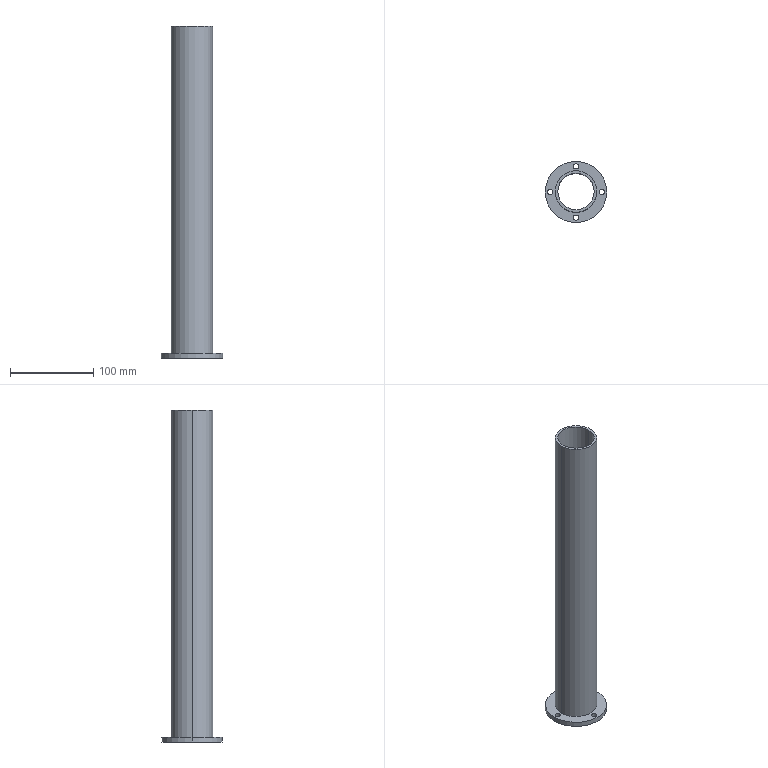Part | STEP file | QA-TE01 | 1 solid | 17 faces | box 74 x 74 x 400 mm | volume 190414 mm3 | cylinder 14 | plane 3 | commonest cylinder face diameters 6.5 x8 44 x2 50 x2 74 x2
STEP:
#1=CARTESIAN_POINT('',(0.,0.,0.));
#2=DIRECTION('',(0.,0.,1.));
#3=DIRECTION('',(1.,0.,0.));
#4=AXIS2_PLACEMENT_3D('',#1,#2,#3);
#5=CARTESIAN_POINT('',(22.,0.,0.));
#6=VERTEX_POINT('',#5);
#7=CARTESIAN_POINT('',(22.,0.,400.));
#8=VERTEX_POINT('',#7);
#9=CARTESIAN_POINT('',(22.,0.,0.));
#10=DIRECTION('',(0.,0.,1.));
#11=VECTOR('',#10,1.);
#12=LINE('',#9,#11);
#13=CARTESIAN_POINT('',(0.,0.,0.));
#14=DIRECTION('',(0.,0.,1.));
#15=DIRECTION('',(1.,0.,0.));
#16=AXIS2_PLACEMENT_3D('',#13,#14,#15);
#17=CYLINDRICAL_SURFACE('',#16,22.);
#18=CARTESIAN_POINT('',(6.283,0.));
#19=DIRECTION('',(0.,1.));
#20=VECTOR('',#19,1.);
#21=LINE('',#18,#20);
#22=(GEOMETRIC_REPRESENTATION_CONTEXT(2)PARAMETRIC_REPRESENTATION_CONTEXT()REPRESENTATION_CONTEXT('',''));
#23=DEFINITIONAL_REPRESENTATION('',(#21),#22);
#24=PCURVE('',#17,#23);
#25=CARTESIAN_POINT('',(0.,0.,0.));
#26=DIRECTION('',(0.,0.,1.));
#27=DIRECTION('',(1.,0.,0.));
#28=AXIS2_PLACEMENT_3D('',#25,#26,#27);
#29=CYLINDRICAL_SURFACE('',#28,22.);
#30=CARTESIAN_POINT('',(0.,0.));
#31=DIRECTION('',(0.,1.));
#32=VECTOR('',#31,1.);
#33=LINE('',#30,#32);
#34=(GEOMETRIC_REPRESENTATION_CONTEXT(2)PARAMETRIC_REPRESENTATION_CONTEXT()REPRESENTATION_CONTEXT('',''));
#35=DEFINITIONAL_REPRESENTATION('',(#33),#34);
#36=PCURVE('',#29,#35);
#37=SURFACE_CURVE('',#12,(#24,#36),.PCURVE_S1.);
#38=EDGE_CURVE('',#6,#8,#37,.T.);
#39=ORIENTED_EDGE('',*,*,#38,.T.);
#40=CARTESIAN_POINT('',(-22.,0.,400.));
#41=VERTEX_POINT('',#40);
#42=CARTESIAN_POINT('',(0.,0.,400.));
#43=DIRECTION('',(0.,0.,1.));
#44=DIRECTION('',(1.,0.,0.));
#45=AXIS2_PLACEMENT_3D('',#42,#43,#44);
#46=CIRCLE('',#45,22.);
#47=CARTESIAN_POINT('',(0.,400.));
#48=DIRECTION('',(1.,0.));
#49=VECTOR('',#48,1.);
#50=LINE('',#47,#49);
#51=(GEOMETRIC_REPRESENTATION_CONTEXT(2)PARAMETRIC_REPRESENTATION_CONTEXT()REPRESENTATION_CONTEXT('',''));
#52=DEFINITIONAL_REPRESENTATION('',(#50),#51);
#53=PCURVE('',#17,#52);
#54=CARTESIAN_POINT('',(0.,0.,400.));
#55=DIRECTION('',(0.,0.,1.));
#56=DIRECTION('',(1.,0.,0.));
#57=AXIS2_PLACEMENT_3D('',#54,#55,#56);
#58=PLANE('',#57);
#59=CARTESIAN_POINT('',(0.,0.));
#60=DIRECTION('',(1.,0.));
#61=AXIS2_PLACEMENT_2D('',#59,#60);
#62=CIRCLE('',#61,22.);
#63=(GEOMETRIC_REPRESENTATION_CONTEXT(2)PARAMETRIC_REPRESENTATION_CONTEXT()REPRESENTATION_CONTEXT('',''));
#64=DEFINITIONAL_REPRESENTATION('',(#62),#63);
#65=PCURVE('',#58,#64);
#66=SURFACE_CURVE('',#46,(#53,#65),.PCURVE_S1.);
#67=EDGE_CURVE('',#41,#8,#66,.T.);
#68=ORIENTED_EDGE('',*,*,#67,.F.);
#69=CARTESIAN_POINT('',(-22.,0.,0.));
#70=VERTEX_POINT('',#69);
#71=CARTESIAN_POINT('',(-22.,0.,0.));
#72=DIRECTION('',(0.,0.,1.));
#73=VECTOR('',#72,1.);
#74=LINE('',#71,#73);
#75=CARTESIAN_POINT('',(3.142,0.));
#76=DIRECTION('',(0.,1.));
#77=VECTOR('',#76,1.);
#78=LINE('',#75,#77);
#79=(GEOMETRIC_REPRESENTATION_CONTEXT(2)PARAMETRIC_REPRESENTATION_CONTEXT()REPRESENTATION_CONTEXT('',''));
#80=DEFINITIONAL_REPRESENTATION('',(#78),#79);
#81=PCURVE('',#17,#80);
#82=CARTESIAN_POINT('',(3.142,0.));
#83=DIRECTION('',(0.,1.));
#84=VECTOR('',#83,1.);
#85=LINE('',#82,#84);
#86=(GEOMETRIC_REPRESENTATION_CONTEXT(2)PARAMETRIC_REPRESENTATION_CONTEXT()REPRESENTATION_CONTEXT('',''));
#87=DEFINITIONAL_REPRESENTATION('',(#85),#86);
#88=PCURVE('',#29,#87);
#89=SURFACE_CURVE('',#74,(#81,#88),.PCURVE_S1.);
#90=EDGE_CURVE('',#70,#41,#89,.T.);
#91=ORIENTED_EDGE('',*,*,#90,.F.);
#92=CARTESIAN_POINT('',(0.,0.,0.));
#93=DIRECTION('',(0.,0.,1.));
#94=DIRECTION('',(1.,0.,0.));
#95=AXIS2_PLACEMENT_3D('',#92,#93,#94);
#96=CIRCLE('',#95,22.);
#97=CARTESIAN_POINT('',(0.,0.));
#98=DIRECTION('',(1.,0.));
#99=VECTOR('',#98,1.);
#100=LINE('',#97,#99);
#101=(GEOMETRIC_REPRESENTATION_CONTEXT(2)PARAMETRIC_REPRESENTATION_CONTEXT()REPRESENTATION_CONTEXT('',''));
#102=DEFINITIONAL_REPRESENTATION('',(#100),#101);
#103=PCURVE('',#17,#102);
#104=CARTESIAN_POINT('',(0.,0.,0.));
#105=DIRECTION('',(0.,0.,1.));
#106=DIRECTION('',(1.,0.,0.));
#107=AXIS2_PLACEMENT_3D('',#104,#105,#106);
#108=PLANE('',#107);
#109=CARTESIAN_POINT('',(0.,0.));
#110=DIRECTION('',(1.,0.));
#111=AXIS2_PLACEMENT_2D('',#109,#110);
#112=CIRCLE('',#111,22.);
#113=(GEOMETRIC_REPRESENTATION_CONTEXT(2)PARAMETRIC_REPRESENTATION_CONTEXT()REPRESENTATION_CONTEXT('',''));
#114=DEFINITIONAL_REPRESENTATION('',(#112),#113);
#115=PCURVE('',#108,#114);
#116=SURFACE_CURVE('',#96,(#103,#115),.PCURVE_S1.);
#117=EDGE_CURVE('',#70,#6,#116,.T.);
#118=ORIENTED_EDGE('',*,*,#117,.T.);
#119=EDGE_LOOP('',(#39,#68,#91,#118));
#120=FACE_BOUND('',#119,.F.);
#121=ADVANCED_FACE('',(#120),#17,.F.);
#122=CARTESIAN_POINT('',(-34.25,0.,6.));
#123=VERTEX_POINT('',#122);
#124=CARTESIAN_POINT('',(-34.25,0.,0.));
#125=VERTEX_POINT('',#124);
#126=CARTESIAN_POINT('',(-34.25,0.,10.));
#127=DIRECTION('',(0.,0.,-1.));
#128=VECTOR('',#127,1.);
#129=LINE('',#126,#128);
#130=CARTESIAN_POINT('',(-31.,0.,10.));
#131=DIRECTION('',(0.,0.,-1.));
#132=DIRECTION('',(-1.,0.,0.));
#133=AXIS2_PLACEMENT_3D('',#130,#131,#132);
#134=CYLINDRICAL_SURFACE('',#133,3.25);
#135=CARTESIAN_POINT('',(6.283,0.));
#136=DIRECTION('',(0.,1.));
#137=VECTOR('',#136,1.);
#138=LINE('',#135,#137);
#139=(GEOMETRIC_REPRESENTATION_CONTEXT(2)PARAMETRIC_REPRESENTATION_CONTEXT()REPRESENTATION_CONTEXT('',''));
#140=DEFINITIONAL_REPRESENTATION('',(#138),#139);
#141=PCURVE('',#134,#140);
#142=CARTESIAN_POINT('',(-31.,0.,10.));
#143=DIRECTION('',(0.,0.,-1.));
#144=DIRECTION('',(-1.,0.,0.));
#145=AXIS2_PLACEMENT_3D('',#142,#143,#144);
#146=CYLINDRICAL_SURFACE('',#145,3.25);
#147=CARTESIAN_POINT('',(0.,0.));
#148=DIRECTION('',(0.,1.));
#149=VECTOR('',#148,1.);
#150=LINE('',#147,#149);
#151=(GEOMETRIC_REPRESENTATION_CONTEXT(2)PARAMETRIC_REPRESENTATION_CONTEXT()REPRESENTATION_CONTEXT('',''));
#152=DEFINITIONAL_REPRESENTATION('',(#150),#151);
#153=PCURVE('',#146,#152);
#154=SURFACE_CURVE('',#129,(#141,#153),.PCURVE_S1.);
#155=EDGE_CURVE('',#123,#125,#154,.T.);
#156=ORIENTED_EDGE('',*,*,#155,.T.);
#157=CARTESIAN_POINT('',(-27.75,0.,0.));
#158=VERTEX_POINT('',#157);
#159=CARTESIAN_POINT('',(-31.,0.,0.));
#160=DIRECTION('',(0.,0.,-1.));
#161=DIRECTION('',(0.,-1.,0.));
#162=AXIS2_PLACEMENT_3D('',#159,#160,#161);
#163=CIRCLE('',#162,3.25);
#164=CARTESIAN_POINT('',(-1.571,10.));
#165=DIRECTION('',(1.,0.));
#166=VECTOR('',#165,1.);
#167=LINE('',#164,#166);
#168=(GEOMETRIC_REPRESENTATION_CONTEXT(2)PARAMETRIC_REPRESENTATION_CONTEXT()REPRESENTATION_CONTEXT('',''));
#169=DEFINITIONAL_REPRESENTATION('',(#167),#168);
#170=PCURVE('',#134,#169);
#171=CARTESIAN_POINT('',(-31.,-3.25));
#172=CARTESIAN_POINT('',(-36.629,-3.25));
#173=CARTESIAN_POINT('',(-33.815,1.625));
#174=CARTESIAN_POINT('',(-31.,6.5));
#175=CARTESIAN_POINT('',(-28.185,1.625));
#176=CARTESIAN_POINT('',(-25.371,-3.25));
#177=CARTESIAN_POINT('',(-31.,-3.25));
#178=(BOUNDED_CURVE()B_SPLINE_CURVE(2,(#171,#172,#173,#174,#175,#176,#177),.UNSPECIFIED.,.T.,.F.)B_SPLINE_CURVE_WITH_KNOTS((1,2,2,2,2,1),(-2.094,0.,2.094,4.189,6.283,8.378),.UNSPECIFIED.)CURVE()GEOMETRIC_REPRESENTATION_ITEM()RATIONAL_B_SPLINE_CURVE((1.,0.5,1.,0.5,1.,0.5,1.))REPRESENTATION_ITEM(''));
#179=(GEOMETRIC_REPRESENTATION_CONTEXT(2)PARAMETRIC_REPRESENTATION_CONTEXT()REPRESENTATION_CONTEXT('',''));
#180=DEFINITIONAL_REPRESENTATION('',(#178),#179);
#181=PCURVE('',#108,#180);
#182=SURFACE_CURVE('',#163,(#170,#181),.PCURVE_S1.);
#183=EDGE_CURVE('',#158,#125,#182,.T.);
#184=ORIENTED_EDGE('',*,*,#183,.F.);
#185=CARTESIAN_POINT('',(-27.75,0.,6.));
#186=VERTEX_POINT('',#185);
#187=CARTESIAN_POINT('',(-27.75,0.,10.));
#188=DIRECTION('',(0.,0.,-1.));
#189=VECTOR('',#188,1.);
#190=LINE('',#187,#189);
#191=CARTESIAN_POINT('',(3.142,0.));
#192=DIRECTION('',(0.,1.));
#193=VECTOR('',#192,1.);
#194=LINE('',#191,#193);
#195=(GEOMETRIC_REPRESENTATION_CONTEXT(2)PARAMETRIC_REPRESENTATION_CONTEXT()REPRESENTATION_CONTEXT('',''));
#196=DEFINITIONAL_REPRESENTATION('',(#194),#195);
#197=PCURVE('',#134,#196);
#198=CARTESIAN_POINT('',(3.142,0.));
#199=DIRECTION('',(0.,1.));
#200=VECTOR('',#199,1.);
#201=LINE('',#198,#200);
#202=(GEOMETRIC_REPRESENTATION_CONTEXT(2)PARAMETRIC_REPRESENTATION_CONTEXT()REPRESENTATION_CONTEXT('',''));
#203=DEFINITIONAL_REPRESENTATION('',(#201),#202);
#204=PCURVE('',#146,#203);
#205=SURFACE_CURVE('',#190,(#197,#204),.PCURVE_S1.);
#206=EDGE_CURVE('',#186,#158,#205,.T.);
#207=ORIENTED_EDGE('',*,*,#206,.F.);
#208=CARTESIAN_POINT('',(-31.,0.,6.));
#209=DIRECTION('',(0.,0.,-1.));
#210=DIRECTION('',(-1.,0.,0.));
#211=AXIS2_PLACEMENT_3D('',#208,#209,#210);
#212=CIRCLE('',#211,3.25);
#213=CARTESIAN_POINT('',(0.,4.));
#214=DIRECTION('',(1.,0.));
#215=VECTOR('',#214,1.);
#216=LINE('',#213,#215);
#217=(GEOMETRIC_REPRESENTATION_CONTEXT(2)PARAMETRIC_REPRESENTATION_CONTEXT()REPRESENTATION_CONTEXT('',''));
#218=DEFINITIONAL_REPRESENTATION('',(#216),#217);
#219=PCURVE('',#134,#218);
#220=CARTESIAN_POINT('',(0.,0.,6.));
#221=DIRECTION('',(0.,0.,-1.));
#222=DIRECTION('',(-1.,0.,0.));
#223=AXIS2_PLACEMENT_3D('',#220,#221,#222);
#224=PLANE('',#223);
#225=CARTESIAN_POINT('',(31.,0.));
#226=DIRECTION('',(1.,0.));
#227=AXIS2_PLACEMENT_2D('',#225,#226);
#228=CIRCLE('',#227,3.25);
#229=(GEOMETRIC_REPRESENTATION_CONTEXT(2)PARAMETRIC_REPRESENTATION_CONTEXT()REPRESENTATION_CONTEXT('',''));
#230=DEFINITIONAL_REPRESENTATION('',(#228),#229);
#231=PCURVE('',#224,#230);
#232=SURFACE_CURVE('',#212,(#219,#231),.PCURVE_S1.);
#233=EDGE_CURVE('',#186,#123,#232,.T.);
#234=ORIENTED_EDGE('',*,*,#233,.T.);
#235=EDGE_LOOP('',(#156,#184,#207,#234));
#236=FACE_BOUND('',#235,.F.);
#237=ADVANCED_FACE('',(#236),#134,.F.);
#238=CARTESIAN_POINT('',(-3.25,-31.,6.));
#239=VERTEX_POINT('',#238);
#240=CARTESIAN_POINT('',(-3.25,-31.,0.));
#241=VERTEX_POINT('',#240);
#242=CARTESIAN_POINT('',(-3.25,-31.,10.));
#243=DIRECTION('',(0.,0.,-1.));
#244=VECTOR('',#243,1.);
#245=LINE('',#242,#244);
#246=CARTESIAN_POINT('',(0.,-31.,10.));
#247=DIRECTION('',(0.,0.,-1.));
#248=DIRECTION('',(-1.,0.,0.));
#249=AXIS2_PLACEMENT_3D('',#246,#247,#248);
#250=CYLINDRICAL_SURFACE('',#249,3.25);
#251=CARTESIAN_POINT('',(6.283,0.));
#252=DIRECTION('',(0.,1.));
#253=VECTOR('',#252,1.);
#254=LINE('',#251,#253);
#255=(GEOMETRIC_REPRESENTATION_CONTEXT(2)PARAMETRIC_REPRESENTATION_CONTEXT()REPRESENTATION_CONTEXT('',''));
#256=DEFINITIONAL_REPRESENTATION('',(#254),#255);
#257=PCURVE('',#250,#256);
#258=CARTESIAN_POINT('',(0.,-31.,10.));
#259=DIRECTION('',(0.,0.,-1.));
#260=DIRECTION('',(-1.,0.,0.));
#261=AXIS2_PLACEMENT_3D('',#258,#259,#260);
#262=CYLINDRICAL_SURFACE('',#261,3.25);
#263=CARTESIAN_POINT('',(0.,0.));
#264=DIRECTION('',(0.,1.));
#265=VECTOR('',#264,1.);
#266=LINE('',#263,#265);
#267=(GEOMETRIC_REPRESENTATION_CONTEXT(2)PARAMETRIC_REPRESENTATION_CONTEXT()REPRESENTATION_CONTEXT('',''));
#268=DEFINITIONAL_REPRESENTATION('',(#266),#267);
#269=PCURVE('',#262,#268);
#270=SURFACE_CURVE('',#245,(#257,#269),.PCURVE_S1.);
#271=EDGE_CURVE('',#239,#241,#270,.T.);
#272=ORIENTED_EDGE('',*,*,#271,.T.);
#273=CARTESIAN_POINT('',(3.25,-31.,0.));
#274=VERTEX_POINT('',#273);
#275=CARTESIAN_POINT('',(0.,-31.,0.));
#276=DIRECTION('',(0.,0.,-1.));
#277=DIRECTION('',(1.,0.,0.));
#278=AXIS2_PLACEMENT_3D('',#275,#276,#277);
#279=CIRCLE('',#278,3.25);
#280=CARTESIAN_POINT('',(3.142,10.));
#281=DIRECTION('',(1.,0.));
#282=VECTOR('',#281,1.);
#283=LINE('',#280,#282);
#284=(GEOMETRIC_REPRESENTATION_CONTEXT(2)PARAMETRIC_REPRESENTATION_CONTEXT()REPRESENTATION_CONTEXT('',''));
#285=DEFINITIONAL_REPRESENTATION('',(#283),#284);
#286=PCURVE('',#250,#285);
#287=CARTESIAN_POINT('',(3.25,-31.));
#288=CARTESIAN_POINT('',(3.25,-36.629));
#289=CARTESIAN_POINT('',(-1.625,-33.815));
#290=CARTESIAN_POINT('',(-6.5,-31.));
#291=CARTESIAN_POINT('',(-1.625,-28.185));
#292=CARTESIAN_POINT('',(3.25,-25.371));
#293=CARTESIAN_POINT('',(3.25,-31.));
#294=(BOUNDED_CURVE()B_SPLINE_CURVE(2,(#287,#288,#289,#290,#291,#292,#293),.UNSPECIFIED.,.T.,.F.)B_SPLINE_CURVE_WITH_KNOTS((1,2,2,2,2,1),(-2.094,0.,2.094,4.189,6.283,8.378),.UNSPECIFIED.)CURVE()GEOMETRIC_REPRESENTATION_ITEM()RATIONAL_B_SPLINE_CURVE((1.,0.5,1.,0.5,1.,0.5,1.))REPRESENTATION_ITEM(''));
#295=(GEOMETRIC_REPRESENTATION_CONTEXT(2)PARAMETRIC_REPRESENTATION_CONTEXT()REPRESENTATION_CONTEXT('',''));
#296=DEFINITIONAL_REPRESENTATION('',(#294),#295);
#297=PCURVE('',#108,#296);
#298=SURFACE_CURVE('',#279,(#286,#297),.PCURVE_S1.);
#299=EDGE_CURVE('',#274,#241,#298,.T.);
#300=ORIENTED_EDGE('',*,*,#299,.F.);
#301=CARTESIAN_POINT('',(3.25,-31.,6.));
#302=VERTEX_POINT('',#301);
#303=CARTESIAN_POINT('',(3.25,-31.,10.));
#304=DIRECTION('',(0.,0.,-1.));
#305=VECTOR('',#304,1.);
#306=LINE('',#303,#305);
#307=CARTESIAN_POINT('',(3.142,0.));
#308=DIRECTION('',(0.,1.));
#309=VECTOR('',#308,1.);
#310=LINE('',#307,#309);
#311=(GEOMETRIC_REPRESENTATION_CONTEXT(2)PARAMETRIC_REPRESENTATION_CONTEXT()REPRESENTATION_CONTEXT('',''));
#312=DEFINITIONAL_REPRESENTATION('',(#310),#311);
#313=PCURVE('',#250,#312);
#314=CARTESIAN_POINT('',(3.142,0.));
#315=DIRECTION('',(0.,1.));
#316=VECTOR('',#315,1.);
#317=LINE('',#314,#316);
#318=(GEOMETRIC_REPRESENTATION_CONTEXT(2)PARAMETRIC_REPRESENTATION_CONTEXT()REPRESENTATION_CONTEXT('',''));
#319=DEFINITIONAL_REPRESENTATION('',(#317),#318);
#320=PCURVE('',#262,#319);
#321=SURFACE_CURVE('',#306,(#313,#320),.PCURVE_S1.);
#322=EDGE_CURVE('',#302,#274,#321,.T.);
#323=ORIENTED_EDGE('',*,*,#322,.F.);
#324=CARTESIAN_POINT('',(0.,-31.,6.));
#325=DIRECTION('',(0.,0.,-1.));
#326=DIRECTION('',(-1.,0.,0.));
#327=AXIS2_PLACEMENT_3D('',#324,#325,#326);
#328=CIRCLE('',#327,3.25);
#329=CARTESIAN_POINT('',(0.,4.));
#330=DIRECTION('',(1.,0.));
#331=VECTOR('',#330,1.);
#332=LINE('',#329,#331);
#333=(GEOMETRIC_REPRESENTATION_CONTEXT(2)PARAMETRIC_REPRESENTATION_CONTEXT()REPRESENTATION_CONTEXT('',''));
#334=DEFINITIONAL_REPRESENTATION('',(#332),#333);
#335=PCURVE('',#250,#334);
#336=CARTESIAN_POINT('',(0.,-31.));
#337=DIRECTION('',(1.,0.));
#338=AXIS2_PLACEMENT_2D('',#336,#337);
#339=CIRCLE('',#338,3.25);
#340=(GEOMETRIC_REPRESENTATION_CONTEXT(2)PARAMETRIC_REPRESENTATION_CONTEXT()REPRESENTATION_CONTEXT('',''));
#341=DEFINITIONAL_REPRESENTATION('',(#339),#340);
#342=PCURVE('',#224,#341);
#343=SURFACE_CURVE('',#328,(#335,#342),.PCURVE_S1.);
#344=EDGE_CURVE('',#302,#239,#343,.T.);
#345=ORIENTED_EDGE('',*,*,#344,.T.);
#346=EDGE_LOOP('',(#272,#300,#323,#345));
#347=FACE_BOUND('',#346,.F.);
#348=ADVANCED_FACE('',(#347),#250,.F.);
#349=CARTESIAN_POINT('',(27.75,0.,6.));
#350=VERTEX_POINT('',#349);
#351=CARTESIAN_POINT('',(27.75,0.,0.));
#352=VERTEX_POINT('',#351);
#353=CARTESIAN_POINT('',(27.75,0.,10.));
#354=DIRECTION('',(0.,0.,-1.));
#355=VECTOR('',#354,1.);
#356=LINE('',#353,#355);
#357=CARTESIAN_POINT('',(31.,0.,10.));
#358=DIRECTION('',(0.,0.,-1.));
#359=DIRECTION('',(-1.,0.,0.));
#360=AXIS2_PLACEMENT_3D('',#357,#358,#359);
#361=CYLINDRICAL_SURFACE('',#360,3.25);
#362=CARTESIAN_POINT('',(6.283,0.));
#363=DIRECTION('',(0.,1.));
#364=VECTOR('',#363,1.);
#365=LINE('',#362,#364);
#366=(GEOMETRIC_REPRESENTATION_CONTEXT(2)PARAMETRIC_REPRESENTATION_CONTEXT()REPRESENTATION_CONTEXT('',''));
#367=DEFINITIONAL_REPRESENTATION('',(#365),#366);
#368=PCURVE('',#361,#367);
#369=CARTESIAN_POINT('',(31.,0.,10.));
#370=DIRECTION('',(0.,0.,-1.));
#371=DIRECTION('',(-1.,0.,0.));
#372=AXIS2_PLACEMENT_3D('',#369,#370,#371);
#373=CYLINDRICAL_SURFACE('',#372,3.25);
#374=CARTESIAN_POINT('',(0.,0.));
#375=DIRECTION('',(0.,1.));
#376=VECTOR('',#375,1.);
#377=LINE('',#374,#376);
#378=(GEOMETRIC_REPRESENTATION_CONTEXT(2)PARAMETRIC_REPRESENTATION_CONTEXT()REPRESENTATION_CONTEXT('',''));
#379=DEFINITIONAL_REPRESENTATION('',(#377),#378);
#380=PCURVE('',#373,#379);
#381=SURFACE_CURVE('',#356,(#368,#380),.PCURVE_S1.);
#382=EDGE_CURVE('',#350,#352,#381,.T.);
#383=ORIENTED_EDGE('',*,*,#382,.T.);
#384=CARTESIAN_POINT('',(34.25,0.,0.));
#385=VERTEX_POINT('',#384);
#386=CARTESIAN_POINT('',(31.,0.,0.));
#387=DIRECTION('',(0.,0.,-1.));
#388=DIRECTION('',(0.,1.,0.));
#389=AXIS2_PLACEMENT_3D('',#386,#387,#388);
#390=CIRCLE('',#389,3.25);
#391=CARTESIAN_POINT('',(1.571,10.));
#392=DIRECTION('',(1.,0.));
#393=VECTOR('',#392,1.);
#394=LINE('',#391,#393);
#395=(GEOMETRIC_REPRESENTATION_CONTEXT(2)PARAMETRIC_REPRESENTATION_CONTEXT()REPRESENTATION_CONTEXT('',''));
#396=DEFINITIONAL_REPRESENTATION('',(#394),#395);
#397=PCURVE('',#361,#396);
#398=CARTESIAN_POINT('',(31.,3.25));
#399=CARTESIAN_POINT('',(36.629,3.25));
#400=CARTESIAN_POINT('',(33.815,-1.625));
#401=CARTESIAN_POINT('',(31.,-6.5));
#402=CARTESIAN_POINT('',(28.185,-1.625));
#403=CARTESIAN_POINT('',(25.371,3.25));
#404=CARTESIAN_POINT('',(31.,3.25));
#405=(BOUNDED_CURVE()B_SPLINE_CURVE(2,(#398,#399,#400,#401,#402,#403,#404),.UNSPECIFIED.,.T.,.F.)B_SPLINE_CURVE_WITH_KNOTS((1,2,2,2,2,1),(-2.094,0.,2.094,4.189,6.283,8.378),.UNSPECIFIED.)CURVE()GEOMETRIC_REPRESENTATION_ITEM()RATIONAL_B_SPLINE_CURVE((1.,0.5,1.,0.5,1.,0.5,1.))REPRESENTATION_ITEM(''));
#406=(GEOMETRIC_REPRESENTATION_CONTEXT(2)PARAMETRIC_REPRESENTATION_CONTEXT()REPRESENTATION_CONTEXT('',''));
#407=DEFINITIONAL_REPRESENTATION('',(#405),#406);
#408=PCURVE('',#108,#407);
#409=SURFACE_CURVE('',#390,(#397,#408),.PCURVE_S1.);
#410=EDGE_CURVE('',#385,#352,#409,.T.);
#411=ORIENTED_EDGE('',*,*,#410,.F.);
#412=CARTESIAN_POINT('',(34.25,0.,6.));
#413=VERTEX_POINT('',#412);
#414=CARTESIAN_POINT('',(34.25,0.,10.));
#415=DIRECTION('',(0.,0.,-1.));
#416=VECTOR('',#415,1.);
#417=LINE('',#414,#416);
#418=CARTESIAN_POINT('',(3.142,0.));
#419=DIRECTION('',(0.,1.));
#420=VECTOR('',#419,1.);
#421=LINE('',#418,#420);
#422=(GEOMETRIC_REPRESENTATION_CONTEXT(2)PARAMETRIC_REPRESENTATION_CONTEXT()REPRESENTATION_CONTEXT('',''));
#423=DEFINITIONAL_REPRESENTATION('',(#421),#422);
#424=PCURVE('',#361,#423);
#425=CARTESIAN_POINT('',(3.142,0.));
#426=DIRECTION('',(0.,1.));
#427=VECTOR('',#426,1.);
#428=LINE('',#425,#427);
#429=(GEOMETRIC_REPRESENTATION_CONTEXT(2)PARAMETRIC_REPRESENTATION_CONTEXT()REPRESENTATION_CONTEXT('',''));
#430=DEFINITIONAL_REPRESENTATION('',(#428),#429);
#431=PCURVE('',#373,#430);
#432=SURFACE_CURVE('',#417,(#424,#431),.PCURVE_S1.);
#433=EDGE_CURVE('',#413,#385,#432,.T.);
#434=ORIENTED_EDGE('',*,*,#433,.F.);
#435=CARTESIAN_POINT('',(31.,0.,6.));
#436=DIRECTION('',(0.,0.,-1.));
#437=DIRECTION('',(-1.,0.,0.));
#438=AXIS2_PLACEMENT_3D('',#435,#436,#437);
#439=CIRCLE('',#438,3.25);
#440=CARTESIAN_POINT('',(0.,4.));
#441=DIRECTION('',(1.,0.));
#442=VECTOR('',#441,1.);
#443=LINE('',#440,#442);
#444=(GEOMETRIC_REPRESENTATION_CONTEXT(2)PARAMETRIC_REPRESENTATION_CONTEXT()REPRESENTATION_CONTEXT('',''));
#445=DEFINITIONAL_REPRESENTATION('',(#443),#444);
#446=PCURVE('',#361,#445);
#447=CARTESIAN_POINT('',(-31.,0.));
#448=DIRECTION('',(1.,0.));
#449=AXIS2_PLACEMENT_2D('',#447,#448);
#450=CIRCLE('',#449,3.25);
#451=(GEOMETRIC_REPRESENTATION_CONTEXT(2)PARAMETRIC_REPRESENTATION_CONTEXT()REPRESENTATION_CONTEXT('',''));
#452=DEFINITIONAL_REPRESENTATION('',(#450),#451);
#453=PCURVE('',#224,#452);
#454=SURFACE_CURVE('',#439,(#446,#453),.PCURVE_S1.);
#455=EDGE_CURVE('',#413,#350,#454,.T.);
#456=ORIENTED_EDGE('',*,*,#455,.T.);
#457=EDGE_LOOP('',(#383,#411,#434,#456));
#458=FACE_BOUND('',#457,.F.);
#459=ADVANCED_FACE('',(#458),#361,.F.);
#460=CARTESIAN_POINT('',(-3.25,31.,6.));
#461=VERTEX_POINT('',#460);
#462=CARTESIAN_POINT('',(-3.25,31.,0.));
#463=VERTEX_POINT('',#462);
#464=CARTESIAN_POINT('',(-3.25,31.,10.));
#465=DIRECTION('',(0.,0.,-1.));
#466=VECTOR('',#465,1.);
#467=LINE('',#464,#466);
#468=CARTESIAN_POINT('',(0.,31.,10.));
#469=DIRECTION('',(0.,0.,-1.));
#470=DIRECTION('',(-1.,0.,0.));
#471=AXIS2_PLACEMENT_3D('',#468,#469,#470);
#472=CYLINDRICAL_SURFACE('',#471,3.25);
#473=CARTESIAN_POINT('',(6.283,0.));
#474=DIRECTION('',(0.,1.));
#475=VECTOR('',#474,1.);
#476=LINE('',#473,#475);
#477=(GEOMETRIC_REPRESENTATION_CONTEXT(2)PARAMETRIC_REPRESENTATION_CONTEXT()REPRESENTATION_CONTEXT('',''));
#478=DEFINITIONAL_REPRESENTATION('',(#476),#477);
#479=PCURVE('',#472,#478);
#480=CARTESIAN_POINT('',(0.,31.,10.));
#481=DIRECTION('',(0.,0.,-1.));
#482=DIRECTION('',(-1.,0.,0.));
#483=AXIS2_PLACEMENT_3D('',#480,#481,#482);
#484=CYLINDRICAL_SURFACE('',#483,3.25);
#485=CARTESIAN_POINT('',(0.,0.));
#486=DIRECTION('',(0.,1.));
#487=VECTOR('',#486,1.);
#488=LINE('',#485,#487);
#489=(GEOMETRIC_REPRESENTATION_CONTEXT(2)PARAMETRIC_REPRESENTATION_CONTEXT()REPRESENTATION_CONTEXT('',''));
#490=DEFINITIONAL_REPRESENTATION('',(#488),#489);
#491=PCURVE('',#484,#490);
#492=SURFACE_CURVE('',#467,(#479,#491),.PCURVE_S1.);
#493=EDGE_CURVE('',#461,#463,#492,.T.);
#494=ORIENTED_EDGE('',*,*,#493,.T.);
#495=CARTESIAN_POINT('',(3.25,31.,0.));
#496=VERTEX_POINT('',#495);
#497=CARTESIAN_POINT('',(0.,31.,0.));
#498=DIRECTION('',(0.,0.,-1.));
#499=DIRECTION('',(-1.,0.,0.));
#500=AXIS2_PLACEMENT_3D('',#497,#498,#499);
#501=CIRCLE('',#500,3.25);
#502=CARTESIAN_POINT('',(0.,10.));
#503=DIRECTION('',(1.,0.));
#504=VECTOR('',#503,1.);
#505=LINE('',#502,#504);
#506=(GEOMETRIC_REPRESENTATION_CONTEXT(2)PARAMETRIC_REPRESENTATION_CONTEXT()REPRESENTATION_CONTEXT('',''));
#507=DEFINITIONAL_REPRESENTATION('',(#505),#506);
#508=PCURVE('',#472,#507);
#509=CARTESIAN_POINT('',(-3.25,31.));
#510=CARTESIAN_POINT('',(-3.25,36.629));
#511=CARTESIAN_POINT('',(1.625,33.815));
#512=CARTESIAN_POINT('',(6.5,31.));
#513=CARTESIAN_POINT('',(1.625,28.185));
#514=CARTESIAN_POINT('',(-3.25,25.371));
#515=CARTESIAN_POINT('',(-3.25,31.));
#516=(BOUNDED_CURVE()B_SPLINE_CURVE(2,(#509,#510,#511,#512,#513,#514,#515),.UNSPECIFIED.,.T.,.F.)B_SPLINE_CURVE_WITH_KNOTS((1,2,2,2,2,1),(-2.094,0.,2.094,4.189,6.283,8.378),.UNSPECIFIED.)CURVE()GEOMETRIC_REPRESENTATION_ITEM()RATIONAL_B_SPLINE_CURVE((1.,0.5,1.,0.5,1.,0.5,1.))REPRESENTATION_ITEM(''));
#517=(GEOMETRIC_REPRESENTATION_CONTEXT(2)PARAMETRIC_REPRESENTATION_CONTEXT()REPRESENTATION_CONTEXT('',''));
#518=DEFINITIONAL_REPRESENTATION('',(#516),#517);
#519=PCURVE('',#108,#518);
#520=SURFACE_CURVE('',#501,(#508,#519),.PCURVE_S1.);
#521=EDGE_CURVE('',#496,#463,#520,.T.);
#522=ORIENTED_EDGE('',*,*,#521,.F.);
#523=CARTESIAN_POINT('',(3.25,31.,6.));
#524=VERTEX_POINT('',#523);
#525=CARTESIAN_POINT('',(3.25,31.,10.));
#526=DIRECTION('',(0.,0.,-1.));
#527=VECTOR('',#526,1.);
#528=LINE('',#525,#527);
#529=CARTESIAN_POINT('',(3.142,0.));
#530=DIRECTION('',(0.,1.));
#531=VECTOR('',#530,1.);
#532=LINE('',#529,#531);
#533=(GEOMETRIC_REPRESENTATION_CONTEXT(2)PARAMETRIC_REPRESENTATION_CONTEXT()REPRESENTATION_CONTEXT('',''));
#534=DEFINITIONAL_REPRESENTATION('',(#532),#533);
#535=PCURVE('',#472,#534);
#536=CARTESIAN_POINT('',(3.142,0.));
#537=DIRECTION('',(0.,1.));
#538=VECTOR('',#537,1.);
#539=LINE('',#536,#538);
#540=(GEOMETRIC_REPRESENTATION_CONTEXT(2)PARAMETRIC_REPRESENTATION_CONTEXT()REPRESENTATION_CONTEXT('',''));
#541=DEFINITIONAL_REPRESENTATION('',(#539),#540);
#542=PCURVE('',#484,#541);
#543=SURFACE_CURVE('',#528,(#535,#542),.PCURVE_S1.);
#544=EDGE_CURVE('',#524,#496,#543,.T.);
#545=ORIENTED_EDGE('',*,*,#544,.F.);
#546=CARTESIAN_POINT('',(0.,31.,6.));
#547=DIRECTION('',(0.,0.,-1.));
#548=DIRECTION('',(-1.,0.,0.));
#549=AXIS2_PLACEMENT_3D('',#546,#547,#548);
#550=CIRCLE('',#549,3.25);
#551=CARTESIAN_POINT('',(0.,4.));
#552=DIRECTION('',(1.,0.));
#553=VECTOR('',#552,1.);
#554=LINE('',#551,#553);
#555=(GEOMETRIC_REPRESENTATION_CONTEXT(2)PARAMETRIC_REPRESENTATION_CONTEXT()REPRESENTATION_CONTEXT('',''));
#556=DEFINITIONAL_REPRESENTATION('',(#554),#555);
#557=PCURVE('',#472,#556);
#558=CARTESIAN_POINT('',(0.,31.));
#559=DIRECTION('',(1.,0.));
#560=AXIS2_PLACEMENT_2D('',#558,#559);
#561=CIRCLE('',#560,3.25);
#562=(GEOMETRIC_REPRESENTATION_CONTEXT(2)PARAMETRIC_REPRESENTATION_CONTEXT()REPRESENTATION_CONTEXT('',''));
#563=DEFINITIONAL_REPRESENTATION('',(#561),#562);
#564=PCURVE('',#224,#563);
#565=SURFACE_CURVE('',#550,(#557,#564),.PCURVE_S1.);
#566=EDGE_CURVE('',#524,#461,#565,.T.);
#567=ORIENTED_EDGE('',*,*,#566,.T.);
#568=EDGE_LOOP('',(#494,#522,#545,#567));
#569=FACE_BOUND('',#568,.F.);
#570=ADVANCED_FACE('',(#569),#472,.F.);
#571=CARTESIAN_POINT('',(-37.,0.,6.));
#572=VERTEX_POINT('',#571);
#573=CARTESIAN_POINT('',(37.,0.,6.));
#574=VERTEX_POINT('',#573);
#575=CARTESIAN_POINT('',(0.,0.,6.));
#576=DIRECTION('',(0.,0.,-1.));
#577=DIRECTION('',(-1.,0.,0.));
#578=AXIS2_PLACEMENT_3D('',#575,#576,#577);
#579=CIRCLE('',#578,37.);
#580=CARTESIAN_POINT('',(0.,0.,6.));
#581=DIRECTION('',(0.,0.,-1.));
#582=DIRECTION('',(-1.,0.,0.));
#583=AXIS2_PLACEMENT_3D('',#580,#581,#582);
#584=CYLINDRICAL_SURFACE('',#583,37.);
#585=CARTESIAN_POINT('',(0.,0.));
#586=DIRECTION('',(1.,0.));
#587=VECTOR('',#586,1.);
#588=LINE('',#585,#587);
#589=(GEOMETRIC_REPRESENTATION_CONTEXT(2)PARAMETRIC_REPRESENTATION_CONTEXT()REPRESENTATION_CONTEXT('',''));
#590=DEFINITIONAL_REPRESENTATION('',(#588),#589);
#591=PCURVE('',#584,#590);
#592=CARTESIAN_POINT('',(0.,0.));
#593=DIRECTION('',(1.,0.));
#594=AXIS2_PLACEMENT_2D('',#592,#593);
#595=CIRCLE('',#594,37.);
#596=(GEOMETRIC_REPRESENTATION_CONTEXT(2)PARAMETRIC_REPRESENTATION_CONTEXT()REPRESENTATION_CONTEXT('',''));
#597=DEFINITIONAL_REPRESENTATION('',(#595),#596);
#598=PCURVE('',#224,#597);
#599=SURFACE_CURVE('',#579,(#591,#598),.PCURVE_S1.);
#600=EDGE_CURVE('',#572,#574,#599,.T.);
#601=ORIENTED_EDGE('',*,*,#600,.T.);
#602=CARTESIAN_POINT('',(37.,0.,0.));
#603=VERTEX_POINT('',#602);
#604=CARTESIAN_POINT('',(37.,0.,6.));
#605=DIRECTION('',(0.,0.,-1.));
#606=VECTOR('',#605,1.);
#607=LINE('',#604,#606);
#608=CARTESIAN_POINT('',(3.142,0.));
#609=DIRECTION('',(0.,1.));
#610=VECTOR('',#609,1.);
#611=LINE('',#608,#610);
#612=(GEOMETRIC_REPRESENTATION_CONTEXT(2)PARAMETRIC_REPRESENTATION_CONTEXT()REPRESENTATION_CONTEXT('',''));
#613=DEFINITIONAL_REPRESENTATION('',(#611),#612);
#614=PCURVE('',#584,#613);
#615=CARTESIAN_POINT('',(0.,0.,6.));
#616=DIRECTION('',(0.,0.,-1.));
#617=DIRECTION('',(-1.,0.,0.));
#618=AXIS2_PLACEMENT_3D('',#615,#616,#617);
#619=CYLINDRICAL_SURFACE('',#618,37.);
#620=CARTESIAN_POINT('',(3.142,0.));
#621=DIRECTION('',(0.,1.));
#622=VECTOR('',#621,1.);
#623=LINE('',#620,#622);
#624=(GEOMETRIC_REPRESENTATION_CONTEXT(2)PARAMETRIC_REPRESENTATION_CONTEXT()REPRESENTATION_CONTEXT('',''));
#625=DEFINITIONAL_REPRESENTATION('',(#623),#624);
#626=PCURVE('',#619,#625);
#627=SURFACE_CURVE('',#607,(#614,#626),.PCURVE_S1.);
#628=EDGE_CURVE('',#574,#603,#627,.T.);
#629=ORIENTED_EDGE('',*,*,#628,.T.);
#630=CARTESIAN_POINT('',(-37.,0.,0.));
#631=VERTEX_POINT('',#630);
#632=CARTESIAN_POINT('',(0.,0.,0.));
#633=DIRECTION('',(0.,0.,-1.));
#634=DIRECTION('',(-1.,0.,0.));
#635=AXIS2_PLACEMENT_3D('',#632,#633,#634);
#636=CIRCLE('',#635,37.);
#637=CARTESIAN_POINT('',(0.,6.));
#638=DIRECTION('',(1.,0.));
#639=VECTOR('',#638,1.);
#640=LINE('',#637,#639);
#641=(GEOMETRIC_REPRESENTATION_CONTEXT(2)PARAMETRIC_REPRESENTATION_CONTEXT()REPRESENTATION_CONTEXT('',''));
#642=DEFINITIONAL_REPRESENTATION('',(#640),#641);
#643=PCURVE('',#584,#642);
#644=CARTESIAN_POINT('',(-37.,0.));
#645=CARTESIAN_POINT('',(-37.,64.086));
#646=CARTESIAN_POINT('',(18.5,32.043));
#647=CARTESIAN_POINT('',(74.,0.));
#648=CARTESIAN_POINT('',(18.5,-32.043));
#649=CARTESIAN_POINT('',(-37.,-64.086));
#650=CARTESIAN_POINT('',(-37.,0.));
#651=(BOUNDED_CURVE()B_SPLINE_CURVE(2,(#644,#645,#646,#647,#648,#649,#650),.UNSPECIFIED.,.T.,.F.)B_SPLINE_CURVE_WITH_KNOTS((1,2,2,2,2,1),(-2.094,0.,2.094,4.189,6.283,8.378),.UNSPECIFIED.)CURVE()GEOMETRIC_REPRESENTATION_ITEM()RATIONAL_B_SPLINE_CURVE((1.,0.5,1.,0.5,1.,0.5,1.))REPRESENTATION_ITEM(''));
#652=(GEOMETRIC_REPRESENTATION_CONTEXT(2)PARAMETRIC_REPRESENTATION_CONTEXT()REPRESENTATION_CONTEXT('',''));
#653=DEFINITIONAL_REPRESENTATION('',(#651),#652);
#654=PCURVE('',#108,#653);
#655=SURFACE_CURVE('',#636,(#643,#654),.PCURVE_S1.);
#656=EDGE_CURVE('',#631,#603,#655,.T.);
#657=ORIENTED_EDGE('',*,*,#656,.F.);
#658=CARTESIAN_POINT('',(-37.,0.,6.));
#659=DIRECTION('',(0.,0.,-1.));
#660=VECTOR('',#659,1.);
#661=LINE('',#658,#660);
#662=CARTESIAN_POINT('',(0.,0.));
#663=DIRECTION('',(0.,1.));
#664=VECTOR('',#663,1.);
#665=LINE('',#662,#664);
#666=(GEOMETRIC_REPRESENTATION_CONTEXT(2)PARAMETRIC_REPRESENTATION_CONTEXT()REPRESENTATION_CONTEXT('',''));
#667=DEFINITIONAL_REPRESENTATION('',(#665),#666);
#668=PCURVE('',#584,#667);
#669=CARTESIAN_POINT('',(6.283,0.));
#670=DIRECTION('',(0.,1.));
#671=VECTOR('',#670,1.);
#672=LINE('',#669,#671);
#673=(GEOMETRIC_REPRESENTATION_CONTEXT(2)PARAMETRIC_REPRESENTATION_CONTEXT()REPRESENTATION_CONTEXT('',''));
#674=DEFINITIONAL_REPRESENTATION('',(#672),#673);
#675=PCURVE('',#619,#674);
#676=SURFACE_CURVE('',#661,(#668,#675),.PCURVE_S1.);
#677=EDGE_CURVE('',#572,#631,#676,.T.);
#678=ORIENTED_EDGE('',*,*,#677,.F.);
#679=EDGE_LOOP('',(#601,#629,#657,#678));
#680=FACE_BOUND('',#679,.T.);
#681=ADVANCED_FACE('',(#680),#584,.T.);
#682=CARTESIAN_POINT('',(25.,0.,400.));
#683=VERTEX_POINT('',#682);
#684=CARTESIAN_POINT('',(-25.,0.,400.));
#685=VERTEX_POINT('',#684);
#686=CARTESIAN_POINT('',(0.,0.,400.));
#687=DIRECTION('',(0.,0.,1.));
#688=DIRECTION('',(1.,0.,0.));
#689=AXIS2_PLACEMENT_3D('',#686,#687,#688);
#690=CIRCLE('',#689,25.);
#691=CARTESIAN_POINT('',(0.,0.,400.));
#692=DIRECTION('',(0.,0.,-1.));
#693=DIRECTION('',(-1.,0.,0.));
#694=AXIS2_PLACEMENT_3D('',#691,#692,#693);
#695=CYLINDRICAL_SURFACE('',#694,25.);
#696=CARTESIAN_POINT('',(3.142,0.));
#697=DIRECTION('',(-1.,0.));
#698=VECTOR('',#697,1.);
#699=LINE('',#696,#698);
#700=(GEOMETRIC_REPRESENTATION_CONTEXT(2)PARAMETRIC_REPRESENTATION_CONTEXT()REPRESENTATION_CONTEXT('',''));
#701=DEFINITIONAL_REPRESENTATION('',(#699),#700);
#702=PCURVE('',#695,#701);
#703=CARTESIAN_POINT('',(0.,0.));
#704=DIRECTION('',(1.,0.));
#705=AXIS2_PLACEMENT_2D('',#703,#704);
#706=CIRCLE('',#705,25.);
#707=(GEOMETRIC_REPRESENTATION_CONTEXT(2)PARAMETRIC_REPRESENTATION_CONTEXT()REPRESENTATION_CONTEXT('',''));
#708=DEFINITIONAL_REPRESENTATION('',(#706),#707);
#709=PCURVE('',#58,#708);
#710=SURFACE_CURVE('',#690,(#702,#709),.PCURVE_S1.);
#711=EDGE_CURVE('',#683,#685,#710,.T.);
#712=ORIENTED_EDGE('',*,*,#711,.F.);
#713=CARTESIAN_POINT('',(25.,0.,6.));
#714=VERTEX_POINT('',#713);
#715=CARTESIAN_POINT('',(25.,0.,400.));
#716=DIRECTION('',(0.,0.,-1.));
#717=VECTOR('',#716,1.);
#718=LINE('',#715,#717);
#719=CARTESIAN_POINT('',(3.142,0.));
#720=DIRECTION('',(0.,1.));
#721=VECTOR('',#720,1.);
#722=LINE('',#719,#721);
#723=(GEOMETRIC_REPRESENTATION_CONTEXT(2)PARAMETRIC_REPRESENTATION_CONTEXT()REPRESENTATION_CONTEXT('',''));
#724=DEFINITIONAL_REPRESENTATION('',(#722),#723);
#725=PCURVE('',#695,#724);
#726=CARTESIAN_POINT('',(0.,0.,400.));
#727=DIRECTION('',(0.,0.,-1.));
#728=DIRECTION('',(-1.,0.,0.));
#729=AXIS2_PLACEMENT_3D('',#726,#727,#728);
#730=CYLINDRICAL_SURFACE('',#729,25.);
#731=CARTESIAN_POINT('',(3.142,0.));
#732=DIRECTION('',(0.,1.));
#733=VECTOR('',#732,1.);
#734=LINE('',#731,#733);
#735=(GEOMETRIC_REPRESENTATION_CONTEXT(2)PARAMETRIC_REPRESENTATION_CONTEXT()REPRESENTATION_CONTEXT('',''));
#736=DEFINITIONAL_REPRESENTATION('',(#734),#735);
#737=PCURVE('',#730,#736);
#738=SURFACE_CURVE('',#718,(#725,#737),.PCURVE_S1.);
#739=EDGE_CURVE('',#683,#714,#738,.T.);
#740=ORIENTED_EDGE('',*,*,#739,.T.);
#741=CARTESIAN_POINT('',(-25.,0.,6.));
#742=VERTEX_POINT('',#741);
#743=CARTESIAN_POINT('',(0.,0.,6.));
#744=DIRECTION('',(0.,0.,-1.));
#745=DIRECTION('',(-1.,0.,0.));
#746=AXIS2_PLACEMENT_3D('',#743,#744,#745);
#747=CIRCLE('',#746,25.);
#748=CARTESIAN_POINT('',(0.,394.));
#749=DIRECTION('',(1.,0.));
#750=VECTOR('',#749,1.);
#751=LINE('',#748,#750);
#752=(GEOMETRIC_REPRESENTATION_CONTEXT(2)PARAMETRIC_REPRESENTATION_CONTEXT()REPRESENTATION_CONTEXT('',''));
#753=DEFINITIONAL_REPRESENTATION('',(#751),#752);
#754=PCURVE('',#695,#753);
#755=CARTESIAN_POINT('',(0.,0.));
#756=DIRECTION('',(1.,0.));
#757=AXIS2_PLACEMENT_2D('',#755,#756);
#758=CIRCLE('',#757,25.);
#759=(GEOMETRIC_REPRESENTATION_CONTEXT(2)PARAMETRIC_REPRESENTATION_CONTEXT()REPRESENTATION_CONTEXT('',''));
#760=DEFINITIONAL_REPRESENTATION('',(#758),#759);
#761=PCURVE('',#224,#760);
#762=SURFACE_CURVE('',#747,(#754,#761),.PCURVE_S1.);
#763=EDGE_CURVE('',#742,#714,#762,.T.);
#764=ORIENTED_EDGE('',*,*,#763,.F.);
#765=CARTESIAN_POINT('',(-25.,0.,400.));
#766=DIRECTION('',(0.,0.,-1.));
#767=VECTOR('',#766,1.);
#768=LINE('',#765,#767);
#769=CARTESIAN_POINT('',(0.,0.));
#770=DIRECTION('',(0.,1.));
#771=VECTOR('',#770,1.);
#772=LINE('',#769,#771);
#773=(GEOMETRIC_REPRESENTATION_CONTEXT(2)PARAMETRIC_REPRESENTATION_CONTEXT()REPRESENTATION_CONTEXT('',''));
#774=DEFINITIONAL_REPRESENTATION('',(#772),#773);
#775=PCURVE('',#695,#774);
#776=CARTESIAN_POINT('',(6.283,0.));
#777=DIRECTION('',(0.,1.));
#778=VECTOR('',#777,1.);
#779=LINE('',#776,#778);
#780=(GEOMETRIC_REPRESENTATION_CONTEXT(2)PARAMETRIC_REPRESENTATION_CONTEXT()REPRESENTATION_CONTEXT('',''));
#781=DEFINITIONAL_REPRESENTATION('',(#779),#780);
#782=PCURVE('',#730,#781);
#783=SURFACE_CURVE('',#768,(#775,#782),.PCURVE_S1.);
#784=EDGE_CURVE('',#685,#742,#783,.T.);
#785=ORIENTED_EDGE('',*,*,#784,.F.);
#786=EDGE_LOOP('',(#712,#740,#764,#785));
#787=FACE_BOUND('',#786,.T.);
#788=ADVANCED_FACE('',(#787),#695,.T.);
#789=ORIENTED_EDGE('',*,*,#739,.F.);
#790=CARTESIAN_POINT('',(0.,0.,400.));
#791=DIRECTION('',(0.,0.,1.));
#792=DIRECTION('',(1.,0.,0.));
#793=AXIS2_PLACEMENT_3D('',#790,#791,#792);
#794=CIRCLE('',#793,25.);
#795=CARTESIAN_POINT('',(9.425,0.));
#796=DIRECTION('',(-1.,0.));
#797=VECTOR('',#796,1.);
#798=LINE('',#795,#797);
#799=(GEOMETRIC_REPRESENTATION_CONTEXT(2)PARAMETRIC_REPRESENTATION_CONTEXT()REPRESENTATION_CONTEXT('',''));
#800=DEFINITIONAL_REPRESENTATION('',(#798),#799);
#801=PCURVE('',#730,#800);
#802=CARTESIAN_POINT('',(0.,0.));
#803=DIRECTION('',(1.,0.));
#804=AXIS2_PLACEMENT_2D('',#802,#803);
#805=CIRCLE('',#804,25.);
#806=(GEOMETRIC_REPRESENTATION_CONTEXT(2)PARAMETRIC_REPRESENTATION_CONTEXT()REPRESENTATION_CONTEXT('',''));
#807=DEFINITIONAL_REPRESENTATION('',(#805),#806);
#808=PCURVE('',#58,#807);
#809=SURFACE_CURVE('',#794,(#801,#808),.PCURVE_S1.);
#810=EDGE_CURVE('',#685,#683,#809,.T.);
#811=ORIENTED_EDGE('',*,*,#810,.F.);
#812=ORIENTED_EDGE('',*,*,#784,.T.);
#813=CARTESIAN_POINT('',(0.,0.,6.));
#814=DIRECTION('',(0.,0.,-1.));
#815=DIRECTION('',(-1.,0.,0.));
#816=AXIS2_PLACEMENT_3D('',#813,#814,#815);
#817=CIRCLE('',#816,25.);
#818=CARTESIAN_POINT('',(0.,394.));
#819=DIRECTION('',(1.,0.));
#820=VECTOR('',#819,1.);
#821=LINE('',#818,#820);
#822=(GEOMETRIC_REPRESENTATION_CONTEXT(2)PARAMETRIC_REPRESENTATION_CONTEXT()REPRESENTATION_CONTEXT('',''));
#823=DEFINITIONAL_REPRESENTATION('',(#821),#822);
#824=PCURVE('',#730,#823);
#825=CARTESIAN_POINT('',(0.,0.));
#826=DIRECTION('',(1.,0.));
#827=AXIS2_PLACEMENT_2D('',#825,#826);
#828=CIRCLE('',#827,25.);
#829=(GEOMETRIC_REPRESENTATION_CONTEXT(2)PARAMETRIC_REPRESENTATION_CONTEXT()REPRESENTATION_CONTEXT('',''));
#830=DEFINITIONAL_REPRESENTATION('',(#828),#829);
#831=PCURVE('',#224,#830);
#832=SURFACE_CURVE('',#817,(#824,#831),.PCURVE_S1.);
#833=EDGE_CURVE('',#714,#742,#832,.T.);
#834=ORIENTED_EDGE('',*,*,#833,.F.);
#835=EDGE_LOOP('',(#789,#811,#812,#834));
#836=FACE_BOUND('',#835,.T.);
#837=ADVANCED_FACE('',(#836),#730,.T.);
#838=CARTESIAN_POINT('',(0.,0.,400.));
#839=DIRECTION('',(0.,0.,1.));
#840=DIRECTION('',(1.,0.,0.));
#841=AXIS2_PLACEMENT_3D('',#838,#839,#840);
#842=CIRCLE('',#841,22.);
#843=CARTESIAN_POINT('',(0.,0.));
#844=DIRECTION('',(1.,0.));
#845=AXIS2_PLACEMENT_2D('',#843,#844);
#846=CIRCLE('',#845,22.);
#847=(GEOMETRIC_REPRESENTATION_CONTEXT(2)PARAMETRIC_REPRESENTATION_CONTEXT()REPRESENTATION_CONTEXT('',''));
#848=DEFINITIONAL_REPRESENTATION('',(#846),#847);
#849=PCURVE('',#58,#848);
#850=CARTESIAN_POINT('',(0.,400.));
#851=DIRECTION('',(1.,0.));
#852=VECTOR('',#851,1.);
#853=LINE('',#850,#852);
#854=(GEOMETRIC_REPRESENTATION_CONTEXT(2)PARAMETRIC_REPRESENTATION_CONTEXT()REPRESENTATION_CONTEXT('',''));
#855=DEFINITIONAL_REPRESENTATION('',(#853),#854);
#856=PCURVE('',#29,#855);
#857=SURFACE_CURVE('',#842,(#849,#856),.PCURVE_S1.);
#858=EDGE_CURVE('',#8,#41,#857,.T.);
#859=ORIENTED_EDGE('',*,*,#858,.F.);
#860=ORIENTED_EDGE('',*,*,#67,.F.);
#861=EDGE_LOOP('',(#859,#860));
#862=FACE_BOUND('',#861,.T.);
#863=ORIENTED_EDGE('',*,*,#810,.T.);
#864=ORIENTED_EDGE('',*,*,#711,.T.);
#865=EDGE_LOOP('',(#863,#864));
#866=FACE_BOUND('',#865,.T.);
#867=ADVANCED_FACE('',(#862,#866),#58,.T.);
#868=CARTESIAN_POINT('',(-31.,0.,6.));
#869=DIRECTION('',(0.,0.,-1.));
#870=DIRECTION('',(-1.,0.,0.));
#871=AXIS2_PLACEMENT_3D('',#868,#869,#870);
#872=CIRCLE('',#871,3.25);
#873=CARTESIAN_POINT('',(31.,0.));
#874=DIRECTION('',(1.,0.));
#875=AXIS2_PLACEMENT_2D('',#873,#874);
#876=CIRCLE('',#875,3.25);
#877=(GEOMETRIC_REPRESENTATION_CONTEXT(2)PARAMETRIC_REPRESENTATION_CONTEXT()REPRESENTATION_CONTEXT('',''));
#878=DEFINITIONAL_REPRESENTATION('',(#876),#877);
#879=PCURVE('',#224,#878);
#880=CARTESIAN_POINT('',(0.,4.));
#881=DIRECTION('',(1.,0.));
#882=VECTOR('',#881,1.);
#883=LINE('',#880,#882);
#884=(GEOMETRIC_REPRESENTATION_CONTEXT(2)PARAMETRIC_REPRESENTATION_CONTEXT()REPRESENTATION_CONTEXT('',''));
#885=DEFINITIONAL_REPRESENTATION('',(#883),#884);
#886=PCURVE('',#146,#885);
#887=SURFACE_CURVE('',#872,(#879,#886),.PCURVE_S1.);
#888=EDGE_CURVE('',#123,#186,#887,.T.);
#889=ORIENTED_EDGE('',*,*,#888,.T.);
#890=ORIENTED_EDGE('',*,*,#233,.T.);
#891=EDGE_LOOP('',(#889,#890));
#892=FACE_BOUND('',#891,.T.);
#893=CARTESIAN_POINT('',(0.,-31.,6.));
#894=DIRECTION('',(0.,0.,-1.));
#895=DIRECTION('',(-1.,0.,0.));
#896=AXIS2_PLACEMENT_3D('',#893,#894,#895);
#897=CIRCLE('',#896,3.25);
#898=CARTESIAN_POINT('',(0.,-31.));
#899=DIRECTION('',(1.,0.));
#900=AXIS2_PLACEMENT_2D('',#898,#899);
#901=CIRCLE('',#900,3.25);
#902=(GEOMETRIC_REPRESENTATION_CONTEXT(2)PARAMETRIC_REPRESENTATION_CONTEXT()REPRESENTATION_CONTEXT('',''));
#903=DEFINITIONAL_REPRESENTATION('',(#901),#902);
#904=PCURVE('',#224,#903);
#905=CARTESIAN_POINT('',(0.,4.));
#906=DIRECTION('',(1.,0.));
#907=VECTOR('',#906,1.);
#908=LINE('',#905,#907);
#909=(GEOMETRIC_REPRESENTATION_CONTEXT(2)PARAMETRIC_REPRESENTATION_CONTEXT()REPRESENTATION_CONTEXT('',''));
#910=DEFINITIONAL_REPRESENTATION('',(#908),#909);
#911=PCURVE('',#262,#910);
#912=SURFACE_CURVE('',#897,(#904,#911),.PCURVE_S1.);
#913=EDGE_CURVE('',#239,#302,#912,.T.);
#914=ORIENTED_EDGE('',*,*,#913,.T.);
#915=ORIENTED_EDGE('',*,*,#344,.T.);
#916=EDGE_LOOP('',(#914,#915));
#917=FACE_BOUND('',#916,.T.);
#918=CARTESIAN_POINT('',(31.,0.,6.));
#919=DIRECTION('',(0.,0.,-1.));
#920=DIRECTION('',(-1.,0.,0.));
#921=AXIS2_PLACEMENT_3D('',#918,#919,#920);
#922=CIRCLE('',#921,3.25);
#923=CARTESIAN_POINT('',(-31.,0.));
#924=DIRECTION('',(1.,0.));
#925=AXIS2_PLACEMENT_2D('',#923,#924);
#926=CIRCLE('',#925,3.25);
#927=(GEOMETRIC_REPRESENTATION_CONTEXT(2)PARAMETRIC_REPRESENTATION_CONTEXT()REPRESENTATION_CONTEXT('',''));
#928=DEFINITIONAL_REPRESENTATION('',(#926),#927);
#929=PCURVE('',#224,#928);
#930=CARTESIAN_POINT('',(0.,4.));
#931=DIRECTION('',(1.,0.));
#932=VECTOR('',#931,1.);
#933=LINE('',#930,#932);
#934=(GEOMETRIC_REPRESENTATION_CONTEXT(2)PARAMETRIC_REPRESENTATION_CONTEXT()REPRESENTATION_CONTEXT('',''));
#935=DEFINITIONAL_REPRESENTATION('',(#933),#934);
#936=PCURVE('',#373,#935);
#937=SURFACE_CURVE('',#922,(#929,#936),.PCURVE_S1.);
#938=EDGE_CURVE('',#350,#413,#937,.T.);
#939=ORIENTED_EDGE('',*,*,#938,.T.);
#940=ORIENTED_EDGE('',*,*,#455,.T.);
#941=EDGE_LOOP('',(#939,#940));
#942=FACE_BOUND('',#941,.T.);
#943=CARTESIAN_POINT('',(0.,31.,6.));
#944=DIRECTION('',(0.,0.,-1.));
#945=DIRECTION('',(-1.,0.,0.));
#946=AXIS2_PLACEMENT_3D('',#943,#944,#945);
#947=CIRCLE('',#946,3.25);
#948=CARTESIAN_POINT('',(0.,31.));
#949=DIRECTION('',(1.,0.));
#950=AXIS2_PLACEMENT_2D('',#948,#949);
#951=CIRCLE('',#950,3.25);
#952=(GEOMETRIC_REPRESENTATION_CONTEXT(2)PARAMETRIC_REPRESENTATION_CONTEXT()REPRESENTATION_CONTEXT('',''));
#953=DEFINITIONAL_REPRESENTATION('',(#951),#952);
#954=PCURVE('',#224,#953);
#955=CARTESIAN_POINT('',(0.,4.));
#956=DIRECTION('',(1.,0.));
#957=VECTOR('',#956,1.);
#958=LINE('',#955,#957);
#959=(GEOMETRIC_REPRESENTATION_CONTEXT(2)PARAMETRIC_REPRESENTATION_CONTEXT()REPRESENTATION_CONTEXT('',''));
#960=DEFINITIONAL_REPRESENTATION('',(#958),#959);
#961=PCURVE('',#484,#960);
#962=SURFACE_CURVE('',#947,(#954,#961),.PCURVE_S1.);
#963=EDGE_CURVE('',#461,#524,#962,.T.);
#964=ORIENTED_EDGE('',*,*,#963,.T.);
#965=ORIENTED_EDGE('',*,*,#566,.T.);
#966=EDGE_LOOP('',(#964,#965));
#967=FACE_BOUND('',#966,.T.);
#968=ORIENTED_EDGE('',*,*,#600,.F.);
#969=CARTESIAN_POINT('',(0.,0.,6.));
#970=DIRECTION('',(0.,0.,-1.));
#971=DIRECTION('',(-1.,0.,0.));
#972=AXIS2_PLACEMENT_3D('',#969,#970,#971);
#973=CIRCLE('',#972,37.);
#974=CARTESIAN_POINT('',(0.,0.));
#975=DIRECTION('',(1.,0.));
#976=AXIS2_PLACEMENT_2D('',#974,#975);
#977=CIRCLE('',#976,37.);
#978=(GEOMETRIC_REPRESENTATION_CONTEXT(2)PARAMETRIC_REPRESENTATION_CONTEXT()REPRESENTATION_CONTEXT('',''));
#979=DEFINITIONAL_REPRESENTATION('',(#977),#978);
#980=PCURVE('',#224,#979);
#981=CARTESIAN_POINT('',(0.,0.));
#982=DIRECTION('',(1.,0.));
#983=VECTOR('',#982,1.);
#984=LINE('',#981,#983);
#985=(GEOMETRIC_REPRESENTATION_CONTEXT(2)PARAMETRIC_REPRESENTATION_CONTEXT()REPRESENTATION_CONTEXT('',''));
#986=DEFINITIONAL_REPRESENTATION('',(#984),#985);
#987=PCURVE('',#619,#986);
#988=SURFACE_CURVE('',#973,(#980,#987),.PCURVE_S1.);
#989=EDGE_CURVE('',#574,#572,#988,.T.);
#990=ORIENTED_EDGE('',*,*,#989,.F.);
#991=EDGE_LOOP('',(#968,#990));
#992=FACE_BOUND('',#991,.T.);
#993=ORIENTED_EDGE('',*,*,#763,.T.);
#994=ORIENTED_EDGE('',*,*,#833,.T.);
#995=EDGE_LOOP('',(#993,#994));
#996=FACE_BOUND('',#995,.T.);
#997=ADVANCED_FACE('',(#892,#917,#942,#967,#992,#996),#224,.F.);
#998=ORIENTED_EDGE('',*,*,#628,.F.);
#999=ORIENTED_EDGE('',*,*,#989,.T.);
#1000=ORIENTED_EDGE('',*,*,#677,.T.);
#1001=CARTESIAN_POINT('',(0.,0.,0.));
#1002=DIRECTION('',(0.,0.,-1.));
#1003=DIRECTION('',(-1.,0.,0.));
#1004=AXIS2_PLACEMENT_3D('',#1001,#1002,#1003);
#1005=CIRCLE('',#1004,37.);
#1006=CARTESIAN_POINT('',(0.,6.));
#1007=DIRECTION('',(1.,0.));
#1008=VECTOR('',#1007,1.);
#1009=LINE('',#1006,#1008);
#1010=(GEOMETRIC_REPRESENTATION_CONTEXT(2)PARAMETRIC_REPRESENTATION_CONTEXT()REPRESENTATION_CONTEXT('',''));
#1011=DEFINITIONAL_REPRESENTATION('',(#1009),#1010);
#1012=PCURVE('',#619,#1011);
#1013=CARTESIAN_POINT('',(-37.,0.));
#1014=CARTESIAN_POINT('',(-37.,64.086));
#1015=CARTESIAN_POINT('',(18.5,32.043));
#1016=CARTESIAN_POINT('',(74.,0.));
#1017=CARTESIAN_POINT('',(18.5,-32.043));
#1018=CARTESIAN_POINT('',(-37.,-64.086));
#1019=CARTESIAN_POINT('',(-37.,0.));
#1020=(BOUNDED_CURVE()B_SPLINE_CURVE(2,(#1013,#1014,#1015,#1016,#1017,#1018,#1019),.UNSPECIFIED.,.T.,.F.)B_SPLINE_CURVE_WITH_KNOTS((1,2,2,2,2,1),(-2.094,0.,2.094,4.189,6.283,8.378),.UNSPECIFIED.)CURVE()GEOMETRIC_REPRESENTATION_ITEM()RATIONAL_B_SPLINE_CURVE((1.,0.5,1.,0.5,1.,0.5,1.))REPRESENTATION_ITEM(''));
#1021=(GEOMETRIC_REPRESENTATION_CONTEXT(2)PARAMETRIC_REPRESENTATION_CONTEXT()REPRESENTATION_CONTEXT('',''));
#1022=DEFINITIONAL_REPRESENTATION('',(#1020),#1021);
#1023=PCURVE('',#108,#1022);
#1024=SURFACE_CURVE('',#1005,(#1012,#1023),.PCURVE_S1.);
#1025=EDGE_CURVE('',#603,#631,#1024,.T.);
#1026=ORIENTED_EDGE('',*,*,#1025,.F.);
#1027=EDGE_LOOP('',(#998,#999,#1000,#1026));
#1028=FACE_BOUND('',#1027,.T.);
#1029=ADVANCED_FACE('',(#1028),#619,.T.);
#1030=CARTESIAN_POINT('',(0.,0.,0.));
#1031=DIRECTION('',(0.,0.,1.));
#1032=DIRECTION('',(1.,0.,0.));
#1033=AXIS2_PLACEMENT_3D('',#1030,#1031,#1032);
#1034=CIRCLE('',#1033,22.);
#1035=CARTESIAN_POINT('',(0.,0.));
#1036=DIRECTION('',(1.,0.));
#1037=AXIS2_PLACEMENT_2D('',#1035,#1036);
#1038=CIRCLE('',#1037,22.);
#1039=(GEOMETRIC_REPRESENTATION_CONTEXT(2)PARAMETRIC_REPRESENTATION_CONTEXT()REPRESENTATION_CONTEXT('',''));
#1040=DEFINITIONAL_REPRESENTATION('',(#1038),#1039);
#1041=PCURVE('',#108,#1040);
#1042=CARTESIAN_POINT('',(0.,0.));
#1043=DIRECTION('',(1.,0.));
#1044=VECTOR('',#1043,1.);
#1045=LINE('',#1042,#1044);
#1046=(GEOMETRIC_REPRESENTATION_CONTEXT(2)PARAMETRIC_REPRESENTATION_CONTEXT()REPRESENTATION_CONTEXT('',''));
#1047=DEFINITIONAL_REPRESENTATION('',(#1045),#1046);
#1048=PCURVE('',#29,#1047);
#1049=SURFACE_CURVE('',#1034,(#1041,#1048),.PCURVE_S1.);
#1050=EDGE_CURVE('',#6,#70,#1049,.T.);
#1051=ORIENTED_EDGE('',*,*,#1050,.T.);
#1052=ORIENTED_EDGE('',*,*,#117,.T.);
#1053=EDGE_LOOP('',(#1051,#1052));
#1054=FACE_BOUND('',#1053,.T.);
#1055=CARTESIAN_POINT('',(-31.,0.,0.));
#1056=DIRECTION('',(0.,0.,-1.));
#1057=DIRECTION('',(0.,-1.,0.));
#1058=AXIS2_PLACEMENT_3D('',#1055,#1056,#1057);
#1059=CIRCLE('',#1058,3.25);
#1060=CARTESIAN_POINT('',(-31.,-3.25));
#1061=CARTESIAN_POINT('',(-36.629,-3.25));
#1062=CARTESIAN_POINT('',(-33.815,1.625));
#1063=CARTESIAN_POINT('',(-31.,6.5));
#1064=CARTESIAN_POINT('',(-28.185,1.625));
#1065=CARTESIAN_POINT('',(-25.371,-3.25));
#1066=CARTESIAN_POINT('',(-31.,-3.25));
#1067=(BOUNDED_CURVE()B_SPLINE_CURVE(2,(#1060,#1061,#1062,#1063,#1064,#1065,#1066),.UNSPECIFIED.,.T.,.F.)B_SPLINE_CURVE_WITH_KNOTS((1,2,2,2,2,1),(-2.094,0.,2.094,4.189,6.283,8.378),.UNSPECIFIED.)CURVE()GEOMETRIC_REPRESENTATION_ITEM()RATIONAL_B_SPLINE_CURVE((1.,0.5,1.,0.5,1.,0.5,1.))REPRESENTATION_ITEM(''));
#1068=(GEOMETRIC_REPRESENTATION_CONTEXT(2)PARAMETRIC_REPRESENTATION_CONTEXT()REPRESENTATION_CONTEXT('',''));
#1069=DEFINITIONAL_REPRESENTATION('',(#1067),#1068);
#1070=PCURVE('',#108,#1069);
#1071=CARTESIAN_POINT('',(-1.571,10.));
#1072=DIRECTION('',(1.,0.));
#1073=VECTOR('',#1072,1.);
#1074=LINE('',#1071,#1073);
#1075=(GEOMETRIC_REPRESENTATION_CONTEXT(2)PARAMETRIC_REPRESENTATION_CONTEXT()REPRESENTATION_CONTEXT('',''));
#1076=DEFINITIONAL_REPRESENTATION('',(#1074),#1075);
#1077=PCURVE('',#146,#1076);
#1078=SURFACE_CURVE('',#1059,(#1070,#1077),.PCURVE_S1.);
#1079=EDGE_CURVE('',#125,#158,#1078,.T.);
#1080=ORIENTED_EDGE('',*,*,#1079,.F.);
#1081=ORIENTED_EDGE('',*,*,#183,.F.);
#1082=EDGE_LOOP('',(#1080,#1081));
#1083=FACE_BOUND('',#1082,.T.);
#1084=CARTESIAN_POINT('',(0.,-31.,0.));
#1085=DIRECTION('',(0.,0.,-1.));
#1086=DIRECTION('',(1.,0.,0.));
#1087=AXIS2_PLACEMENT_3D('',#1084,#1085,#1086);
#1088=CIRCLE('',#1087,3.25);
#1089=CARTESIAN_POINT('',(3.25,-31.));
#1090=CARTESIAN_POINT('',(3.25,-36.629));
#1091=CARTESIAN_POINT('',(-1.625,-33.815));
#1092=CARTESIAN_POINT('',(-6.5,-31.));
#1093=CARTESIAN_POINT('',(-1.625,-28.185));
#1094=CARTESIAN_POINT('',(3.25,-25.371));
#1095=CARTESIAN_POINT('',(3.25,-31.));
#1096=(BOUNDED_CURVE()B_SPLINE_CURVE(2,(#1089,#1090,#1091,#1092,#1093,#1094,#1095),.UNSPECIFIED.,.T.,.F.)B_SPLINE_CURVE_WITH_KNOTS((1,2,2,2,2,1),(-2.094,0.,2.094,4.189,6.283,8.378),.UNSPECIFIED.)CURVE()GEOMETRIC_REPRESENTATION_ITEM()RATIONAL_B_SPLINE_CURVE((1.,0.5,1.,0.5,1.,0.5,1.))REPRESENTATION_ITEM(''));
#1097=(GEOMETRIC_REPRESENTATION_CONTEXT(2)PARAMETRIC_REPRESENTATION_CONTEXT()REPRESENTATION_CONTEXT('',''));
#1098=DEFINITIONAL_REPRESENTATION('',(#1096),#1097);
#1099=PCURVE('',#108,#1098);
#1100=CARTESIAN_POINT('',(-3.142,10.));
#1101=DIRECTION('',(1.,0.));
#1102=VECTOR('',#1101,1.);
#1103=LINE('',#1100,#1102);
#1104=(GEOMETRIC_REPRESENTATION_CONTEXT(2)PARAMETRIC_REPRESENTATION_CONTEXT()REPRESENTATION_CONTEXT('',''));
#1105=DEFINITIONAL_REPRESENTATION('',(#1103),#1104);
#1106=PCURVE('',#262,#1105);
#1107=SURFACE_CURVE('',#1088,(#1099,#1106),.PCURVE_S1.);
#1108=EDGE_CURVE('',#241,#274,#1107,.T.);
#1109=ORIENTED_EDGE('',*,*,#1108,.F.);
#1110=ORIENTED_EDGE('',*,*,#299,.F.);
#1111=EDGE_LOOP('',(#1109,#1110));
#1112=FACE_BOUND('',#1111,.T.);
#1113=CARTESIAN_POINT('',(31.,0.,0.));
#1114=DIRECTION('',(0.,0.,-1.));
#1115=DIRECTION('',(0.,1.,0.));
#1116=AXIS2_PLACEMENT_3D('',#1113,#1114,#1115);
#1117=CIRCLE('',#1116,3.25);
#1118=CARTESIAN_POINT('',(31.,3.25));
#1119=CARTESIAN_POINT('',(36.629,3.25));
#1120=CARTESIAN_POINT('',(33.815,-1.625));
#1121=CARTESIAN_POINT('',(31.,-6.5));
#1122=CARTESIAN_POINT('',(28.185,-1.625));
#1123=CARTESIAN_POINT('',(25.371,3.25));
#1124=CARTESIAN_POINT('',(31.,3.25));
#1125=(BOUNDED_CURVE()B_SPLINE_CURVE(2,(#1118,#1119,#1120,#1121,#1122,#1123,#1124),.UNSPECIFIED.,.T.,.F.)B_SPLINE_CURVE_WITH_KNOTS((1,2,2,2,2,1),(-2.094,0.,2.094,4.189,6.283,8.378),.UNSPECIFIED.)CURVE()GEOMETRIC_REPRESENTATION_ITEM()RATIONAL_B_SPLINE_CURVE((1.,0.5,1.,0.5,1.,0.5,1.))REPRESENTATION_ITEM(''));
#1126=(GEOMETRIC_REPRESENTATION_CONTEXT(2)PARAMETRIC_REPRESENTATION_CONTEXT()REPRESENTATION_CONTEXT('',''));
#1127=DEFINITIONAL_REPRESENTATION('',(#1125),#1126);
#1128=PCURVE('',#108,#1127);
#1129=CARTESIAN_POINT('',(-4.712,10.));
#1130=DIRECTION('',(1.,0.));
#1131=VECTOR('',#1130,1.);
#1132=LINE('',#1129,#1131);
#1133=(GEOMETRIC_REPRESENTATION_CONTEXT(2)PARAMETRIC_REPRESENTATION_CONTEXT()REPRESENTATION_CONTEXT('',''));
#1134=DEFINITIONAL_REPRESENTATION('',(#1132),#1133);
#1135=PCURVE('',#373,#1134);
#1136=SURFACE_CURVE('',#1117,(#1128,#1135),.PCURVE_S1.);
#1137=EDGE_CURVE('',#352,#385,#1136,.T.);
#1138=ORIENTED_EDGE('',*,*,#1137,.F.);
#1139=ORIENTED_EDGE('',*,*,#410,.F.);
#1140=EDGE_LOOP('',(#1138,#1139));
#1141=FACE_BOUND('',#1140,.T.);
#1142=CARTESIAN_POINT('',(0.,31.,0.));
#1143=DIRECTION('',(0.,0.,-1.));
#1144=DIRECTION('',(-1.,0.,0.));
#1145=AXIS2_PLACEMENT_3D('',#1142,#1143,#1144);
#1146=CIRCLE('',#1145,3.25);
#1147=CARTESIAN_POINT('',(-3.25,31.));
#1148=CARTESIAN_POINT('',(-3.25,36.629));
#1149=CARTESIAN_POINT('',(1.625,33.815));
#1150=CARTESIAN_POINT('',(6.5,31.));
#1151=CARTESIAN_POINT('',(1.625,28.185));
#1152=CARTESIAN_POINT('',(-3.25,25.371));
#1153=CARTESIAN_POINT('',(-3.25,31.));
#1154=(BOUNDED_CURVE()B_SPLINE_CURVE(2,(#1147,#1148,#1149,#1150,#1151,#1152,#1153),.UNSPECIFIED.,.T.,.F.)B_SPLINE_CURVE_WITH_KNOTS((1,2,2,2,2,1),(-2.094,0.,2.094,4.189,6.283,8.378),.UNSPECIFIED.)CURVE()GEOMETRIC_REPRESENTATION_ITEM()RATIONAL_B_SPLINE_CURVE((1.,0.5,1.,0.5,1.,0.5,1.))REPRESENTATION_ITEM(''));
#1155=(GEOMETRIC_REPRESENTATION_CONTEXT(2)PARAMETRIC_REPRESENTATION_CONTEXT()REPRESENTATION_CONTEXT('',''));
#1156=DEFINITIONAL_REPRESENTATION('',(#1154),#1155);
#1157=PCURVE('',#108,#1156);
#1158=CARTESIAN_POINT('',(0.,10.));
#1159=DIRECTION('',(1.,0.));
#1160=VECTOR('',#1159,1.);
#1161=LINE('',#1158,#1160);
#1162=(GEOMETRIC_REPRESENTATION_CONTEXT(2)PARAMETRIC_REPRESENTATION_CONTEXT()REPRESENTATION_CONTEXT('',''));
#1163=DEFINITIONAL_REPRESENTATION('',(#1161),#1162);
#1164=PCURVE('',#484,#1163);
#1165=SURFACE_CURVE('',#1146,(#1157,#1164),.PCURVE_S1.);
#1166=EDGE_CURVE('',#463,#496,#1165,.T.);
#1167=ORIENTED_EDGE('',*,*,#1166,.F.);
#1168=ORIENTED_EDGE('',*,*,#521,.F.);
#1169=EDGE_LOOP('',(#1167,#1168));
#1170=FACE_BOUND('',#1169,.T.);
#1171=ORIENTED_EDGE('',*,*,#656,.T.);
#1172=ORIENTED_EDGE('',*,*,#1025,.T.);
#1173=EDGE_LOOP('',(#1171,#1172));
#1174=FACE_BOUND('',#1173,.T.);
#1175=ADVANCED_FACE('',(#1054,#1083,#1112,#1141,#1170,#1174),#108,.F.);
#1176=ORIENTED_EDGE('',*,*,#1166,.F.);
#1177=ORIENTED_EDGE('',*,*,#493,.F.);
#1178=ORIENTED_EDGE('',*,*,#963,.T.);
#1179=ORIENTED_EDGE('',*,*,#544,.T.);
#1180=EDGE_LOOP('',(#1176,#1177,#1178,#1179));
#1181=FACE_BOUND('',#1180,.F.);
#1182=ADVANCED_FACE('',(#1181),#484,.F.);
#1183=ORIENTED_EDGE('',*,*,#1137,.F.);
#1184=ORIENTED_EDGE('',*,*,#382,.F.);
#1185=ORIENTED_EDGE('',*,*,#938,.T.);
#1186=ORIENTED_EDGE('',*,*,#433,.T.);
#1187=EDGE_LOOP('',(#1183,#1184,#1185,#1186));
#1188=FACE_BOUND('',#1187,.F.);
#1189=ADVANCED_FACE('',(#1188),#373,.F.);
#1190=ORIENTED_EDGE('',*,*,#1108,.F.);
#1191=ORIENTED_EDGE('',*,*,#271,.F.);
#1192=ORIENTED_EDGE('',*,*,#913,.T.);
#1193=ORIENTED_EDGE('',*,*,#322,.T.);
#1194=EDGE_LOOP('',(#1190,#1191,#1192,#1193));
#1195=FACE_BOUND('',#1194,.F.);
#1196=ADVANCED_FACE('',(#1195),#262,.F.);
#1197=ORIENTED_EDGE('',*,*,#1079,.F.);
#1198=ORIENTED_EDGE('',*,*,#155,.F.);
#1199=ORIENTED_EDGE('',*,*,#888,.T.);
#1200=ORIENTED_EDGE('',*,*,#206,.T.);
#1201=EDGE_LOOP('',(#1197,#1198,#1199,#1200));
#1202=FACE_BOUND('',#1201,.F.);
#1203=ADVANCED_FACE('',(#1202),#146,.F.);
#1204=ORIENTED_EDGE('',*,*,#858,.F.);
#1205=ORIENTED_EDGE('',*,*,#38,.F.);
#1206=ORIENTED_EDGE('',*,*,#1050,.T.);
#1207=ORIENTED_EDGE('',*,*,#90,.T.);
#1208=EDGE_LOOP('',(#1204,#1205,#1206,#1207));
#1209=FACE_BOUND('',#1208,.F.);
#1210=ADVANCED_FACE('',(#1209),#29,.F.);
#1211=CLOSED_SHELL('',(#121,#237,#348,#459,#570,#681,#788,#837,#867,#997,#1029,#1175,#1182,#1189,#1196,#1203,#1210));
#1212=MANIFOLD_SOLID_BREP('',#1211);
#1213=(LENGTH_UNIT()NAMED_UNIT(*)SI_UNIT(.MILLI.,.METRE.));
#1214=UNCERTAINTY_MEASURE_WITH_UNIT(LENGTH_MEASURE(0.0000001),#1213,'','');
#1215=(NAMED_UNIT(*)PLANE_ANGLE_UNIT()SI_UNIT($,.RADIAN.));
#1216=(NAMED_UNIT(*)SI_UNIT($,.STERADIAN.)SOLID_ANGLE_UNIT());
#1217=(GEOMETRIC_REPRESENTATION_CONTEXT(3)GLOBAL_UNCERTAINTY_ASSIGNED_CONTEXT((#1214))GLOBAL_UNIT_ASSIGNED_CONTEXT((#1213,#1215,#1216))REPRESENTATION_CONTEXT('',''));
#1218=ADVANCED_BREP_SHAPE_REPRESENTATION('',(#4,#1212),#1217);